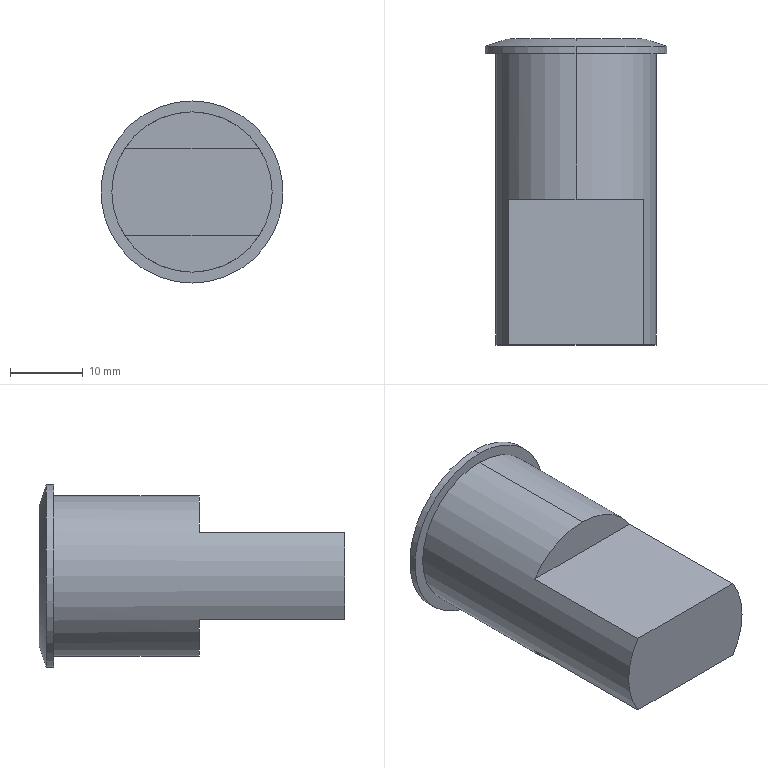Part | SolidWorks | features ICE 2, Chamfer 1, Extrusion 1 | 1 solid | 13 faces | box 25 x 42 x 25 mm | volume 13481 mm3 | plane 7 | cylinder 4 | cone 2 | commonest cylinder face diameters 22 x2 25 x2
STEP:
#1=CARTESIAN_POINT('',(0.,22.,9.5));
#2=VERTEX_POINT('',#1);
#3=CARTESIAN_POINT('',(0.,22.,-9.5));
#4=VERTEX_POINT('',#3);
#5=CARTESIAN_POINT('',(0.,22.,0.));
#6=DIRECTION('',(0.,1.,0.));
#7=DIRECTION('',(0.,0.,1.));
#8=AXIS2_PLACEMENT_3D('',#5,#6,#7);
#9=CIRCLE('',#8,9.5);
#10=EDGE_CURVE('',#2,#4,#9,.T.);
#11=ORIENTED_EDGE('',*,*,#10,.F.);
#12=CARTESIAN_POINT('',(0.,21.,12.5));
#13=VERTEX_POINT('',#12);
#14=CARTESIAN_POINT('',(0.,22.,9.5));
#15=DIRECTION('',(0.,-0.3162,0.9487));
#16=VECTOR('',#15,1000.);
#17=LINE('',#14,#16);
#18=EDGE_CURVE('',#2,#13,#17,.T.);
#19=ORIENTED_EDGE('',*,*,#18,.T.);
#20=CARTESIAN_POINT('',(0.,21.,-12.5));
#21=VERTEX_POINT('',#20);
#22=CARTESIAN_POINT('',(0.,21.,0.));
#23=DIRECTION('',(0.,-1.,0.));
#24=DIRECTION('',(0.,0.,1.));
#25=AXIS2_PLACEMENT_3D('',#22,#23,#24);
#26=CIRCLE('',#25,12.5);
#27=EDGE_CURVE('',#21,#13,#26,.T.);
#28=ORIENTED_EDGE('',*,*,#27,.F.);
#29=CARTESIAN_POINT('',(0.,22.,-9.5));
#30=DIRECTION('',(0.,-0.3162,-0.9487));
#31=VECTOR('',#30,1000.);
#32=LINE('',#29,#31);
#33=EDGE_CURVE('',#4,#21,#32,.T.);
#34=ORIENTED_EDGE('',*,*,#33,.F.);
#35=EDGE_LOOP('',(#11,#19,#28,#34));
#36=FACE_OUTER_BOUND('',#35,.T.);
#37=CARTESIAN_POINT('',(0.,22.,0.));
#38=DIRECTION('',(0.,-1.,0.));
#39=DIRECTION('',(0.,0.,-1.));
#40=AXIS2_PLACEMENT_3D('',#37,#38,#39);
#41=CONICAL_SURFACE('',#40,9.5,1.249);
#42=ADVANCED_FACE('',(#36),#41,.T.);
#43=ORIENTED_EDGE('',*,*,#27,.T.);
#44=CARTESIAN_POINT('',(0.,20.,12.5));
#45=VERTEX_POINT('',#44);
#46=CARTESIAN_POINT('',(0.,22.,12.5));
#47=DIRECTION('',(0.,-1.,0.));
#48=VECTOR('',#47,1000.);
#49=LINE('',#46,#48);
#50=EDGE_CURVE('',#13,#45,#49,.T.);
#51=ORIENTED_EDGE('',*,*,#50,.T.);
#52=CARTESIAN_POINT('',(0.,20.,-12.5));
#53=VERTEX_POINT('',#52);
#54=CARTESIAN_POINT('',(0.,20.,0.));
#55=DIRECTION('',(0.,1.,0.));
#56=DIRECTION('',(0.,0.,1.));
#57=AXIS2_PLACEMENT_3D('',#54,#55,#56);
#58=CIRCLE('',#57,12.5);
#59=EDGE_CURVE('',#45,#53,#58,.T.);
#60=ORIENTED_EDGE('',*,*,#59,.T.);
#61=CARTESIAN_POINT('',(0.,22.,-12.5));
#62=DIRECTION('',(0.,-1.,0.));
#63=VECTOR('',#62,1000.);
#64=LINE('',#61,#63);
#65=EDGE_CURVE('',#21,#53,#64,.T.);
#66=ORIENTED_EDGE('',*,*,#65,.F.);
#67=EDGE_LOOP('',(#43,#51,#60,#66));
#68=FACE_OUTER_BOUND('',#67,.T.);
#69=CARTESIAN_POINT('',(0.,22.,0.));
#70=DIRECTION('',(0.,-1.,0.));
#71=DIRECTION('',(0.,0.,-1.));
#72=AXIS2_PLACEMENT_3D('',#69,#70,#71);
#73=CYLINDRICAL_SURFACE('',#72,12.5);
#74=ADVANCED_FACE('',(#68),#73,.T.);
#75=CARTESIAN_POINT('',(0.,20.,11.));
#76=VERTEX_POINT('',#75);
#77=CARTESIAN_POINT('',(0.,20.,-11.));
#78=VERTEX_POINT('',#77);
#79=CARTESIAN_POINT('',(0.,20.,0.));
#80=DIRECTION('',(0.,1.,0.));
#81=DIRECTION('',(0.,0.,1.));
#82=AXIS2_PLACEMENT_3D('',#79,#80,#81);
#83=CIRCLE('',#82,11.);
#84=EDGE_CURVE('',#76,#78,#83,.T.);
#85=ORIENTED_EDGE('',*,*,#84,.F.);
#86=CARTESIAN_POINT('',(0.,0.,11.));
#87=VERTEX_POINT('',#86);
#88=CARTESIAN_POINT('',(0.,20.,11.));
#89=DIRECTION('',(0.,-1.,0.));
#90=VECTOR('',#89,1000.);
#91=LINE('',#88,#90);
#92=EDGE_CURVE('',#76,#87,#91,.T.);
#93=ORIENTED_EDGE('',*,*,#92,.T.);
#94=CARTESIAN_POINT('',(9.22,0.,6.));
#95=VERTEX_POINT('',#94);
#96=CARTESIAN_POINT('',(0.,0.,0.));
#97=DIRECTION('',(0.,1.,0.));
#98=DIRECTION('',(0.,0.,1.));
#99=AXIS2_PLACEMENT_3D('',#96,#97,#98);
#100=CIRCLE('',#99,11.);
#101=EDGE_CURVE('',#87,#95,#100,.T.);
#102=ORIENTED_EDGE('',*,*,#101,.T.);
#103=CARTESIAN_POINT('',(9.22,-20.,6.));
#104=VERTEX_POINT('',#103);
#105=CARTESIAN_POINT('',(9.22,-20.,6.));
#106=DIRECTION('',(0.,1.,0.));
#107=VECTOR('',#106,1000.);
#108=LINE('',#105,#107);
#109=EDGE_CURVE('',#104,#95,#108,.T.);
#110=ORIENTED_EDGE('',*,*,#109,.F.);
#111=CARTESIAN_POINT('',(9.22,-20.,-6.));
#112=VERTEX_POINT('',#111);
#113=CARTESIAN_POINT('',(0.,-20.,0.));
#114=DIRECTION('',(0.,-1.,0.));
#115=DIRECTION('',(0.,0.,-1.));
#116=AXIS2_PLACEMENT_3D('',#113,#114,#115);
#117=CIRCLE('',#116,11.);
#118=EDGE_CURVE('',#112,#104,#117,.T.);
#119=ORIENTED_EDGE('',*,*,#118,.F.);
#120=CARTESIAN_POINT('',(9.22,0.,-6.));
#121=VERTEX_POINT('',#120);
#122=CARTESIAN_POINT('',(9.22,-20.,-6.));
#123=DIRECTION('',(0.,1.,0.));
#124=VECTOR('',#123,1000.);
#125=LINE('',#122,#124);
#126=EDGE_CURVE('',#112,#121,#125,.T.);
#127=ORIENTED_EDGE('',*,*,#126,.T.);
#128=CARTESIAN_POINT('',(0.,0.,-11.));
#129=VERTEX_POINT('',#128);
#130=CARTESIAN_POINT('',(0.,0.,0.));
#131=DIRECTION('',(0.,1.,0.));
#132=DIRECTION('',(0.,0.,1.));
#133=AXIS2_PLACEMENT_3D('',#130,#131,#132);
#134=CIRCLE('',#133,11.);
#135=EDGE_CURVE('',#121,#129,#134,.T.);
#136=ORIENTED_EDGE('',*,*,#135,.T.);
#137=CARTESIAN_POINT('',(0.,20.,-11.));
#138=DIRECTION('',(0.,-1.,0.));
#139=VECTOR('',#138,1000.);
#140=LINE('',#137,#139);
#141=EDGE_CURVE('',#78,#129,#140,.T.);
#142=ORIENTED_EDGE('',*,*,#141,.F.);
#143=EDGE_LOOP('',(#85,#93,#102,#110,#119,#127,#136,#142));
#144=FACE_OUTER_BOUND('',#143,.T.);
#145=CARTESIAN_POINT('',(0.,20.,0.));
#146=DIRECTION('',(0.,-1.,0.));
#147=DIRECTION('',(0.,0.,-1.));
#148=AXIS2_PLACEMENT_3D('',#145,#146,#147);
#149=CYLINDRICAL_SURFACE('',#148,11.);
#150=ADVANCED_FACE('',(#144),#149,.T.);
#151=CARTESIAN_POINT('',(-9.22,0.,-6.));
#152=VERTEX_POINT('',#151);
#153=CARTESIAN_POINT('',(0.,0.,-6.));
#154=DIRECTION('',(1.,0.,0.));
#155=VECTOR('',#154,1000.);
#156=LINE('',#153,#155);
#157=EDGE_CURVE('',#152,#121,#156,.T.);
#158=ORIENTED_EDGE('',*,*,#157,.F.);
#159=CARTESIAN_POINT('',(0.,0.,0.));
#160=DIRECTION('',(0.,1.,0.));
#161=DIRECTION('',(0.,0.,1.));
#162=AXIS2_PLACEMENT_3D('',#159,#160,#161);
#163=CIRCLE('',#162,11.);
#164=EDGE_CURVE('',#129,#152,#163,.T.);
#165=ORIENTED_EDGE('',*,*,#164,.F.);
#166=ORIENTED_EDGE('',*,*,#135,.F.);
#167=EDGE_LOOP('',(#158,#165,#166));
#168=FACE_OUTER_BOUND('',#167,.T.);
#169=CARTESIAN_POINT('',(0.,0.,0.));
#170=DIRECTION('',(0.,1.,0.));
#171=DIRECTION('',(0.,0.,1.));
#172=AXIS2_PLACEMENT_3D('',#169,#170,#171);
#173=PLANE('',#172);
#174=ADVANCED_FACE('',(#168),#173,.F.);
#175=ORIENTED_EDGE('',*,*,#92,.F.);
#176=CARTESIAN_POINT('',(0.,20.,0.));
#177=DIRECTION('',(0.,1.,0.));
#178=DIRECTION('',(0.,0.,1.));
#179=AXIS2_PLACEMENT_3D('',#176,#177,#178);
#180=CIRCLE('',#179,11.);
#181=EDGE_CURVE('',#78,#76,#180,.T.);
#182=ORIENTED_EDGE('',*,*,#181,.F.);
#183=ORIENTED_EDGE('',*,*,#141,.T.);
#184=ORIENTED_EDGE('',*,*,#164,.T.);
#185=CARTESIAN_POINT('',(-9.22,-20.,-6.));
#186=VERTEX_POINT('',#185);
#187=CARTESIAN_POINT('',(-9.22,-20.,-6.));
#188=DIRECTION('',(0.,1.,0.));
#189=VECTOR('',#188,1000.);
#190=LINE('',#187,#189);
#191=EDGE_CURVE('',#186,#152,#190,.T.);
#192=ORIENTED_EDGE('',*,*,#191,.F.);
#193=CARTESIAN_POINT('',(-9.22,-20.,6.));
#194=VERTEX_POINT('',#193);
#195=CARTESIAN_POINT('',(0.,-20.,0.));
#196=DIRECTION('',(0.,-1.,0.));
#197=DIRECTION('',(0.,0.,-1.));
#198=AXIS2_PLACEMENT_3D('',#195,#196,#197);
#199=CIRCLE('',#198,11.);
#200=EDGE_CURVE('',#194,#186,#199,.T.);
#201=ORIENTED_EDGE('',*,*,#200,.F.);
#202=CARTESIAN_POINT('',(-9.22,0.,6.));
#203=VERTEX_POINT('',#202);
#204=CARTESIAN_POINT('',(-9.22,-20.,6.));
#205=DIRECTION('',(0.,1.,0.));
#206=VECTOR('',#205,1000.);
#207=LINE('',#204,#206);
#208=EDGE_CURVE('',#194,#203,#207,.T.);
#209=ORIENTED_EDGE('',*,*,#208,.T.);
#210=CARTESIAN_POINT('',(0.,0.,0.));
#211=DIRECTION('',(0.,1.,0.));
#212=DIRECTION('',(0.,0.,1.));
#213=AXIS2_PLACEMENT_3D('',#210,#211,#212);
#214=CIRCLE('',#213,11.);
#215=EDGE_CURVE('',#203,#87,#214,.T.);
#216=ORIENTED_EDGE('',*,*,#215,.T.);
#217=EDGE_LOOP('',(#175,#182,#183,#184,#192,#201,#209,#216));
#218=FACE_OUTER_BOUND('',#217,.T.);
#219=CARTESIAN_POINT('',(0.,20.,0.));
#220=DIRECTION('',(0.,-1.,0.));
#221=DIRECTION('',(0.,0.,-1.));
#222=AXIS2_PLACEMENT_3D('',#219,#220,#221);
#223=CYLINDRICAL_SURFACE('',#222,11.);
#224=ADVANCED_FACE('',(#218),#223,.T.);
#225=ORIENTED_EDGE('',*,*,#215,.F.);
#226=CARTESIAN_POINT('',(0.,0.,6.));
#227=DIRECTION('',(1.,0.,0.));
#228=VECTOR('',#227,1000.);
#229=LINE('',#226,#228);
#230=EDGE_CURVE('',#203,#95,#229,.T.);
#231=ORIENTED_EDGE('',*,*,#230,.T.);
#232=ORIENTED_EDGE('',*,*,#101,.F.);
#233=EDGE_LOOP('',(#225,#231,#232));
#234=FACE_OUTER_BOUND('',#233,.T.);
#235=CARTESIAN_POINT('',(0.,0.,0.));
#236=DIRECTION('',(0.,1.,0.));
#237=DIRECTION('',(0.,0.,1.));
#238=AXIS2_PLACEMENT_3D('',#235,#236,#237);
#239=PLANE('',#238);
#240=ADVANCED_FACE('',(#234),#239,.F.);
#241=ORIENTED_EDGE('',*,*,#157,.T.);
#242=ORIENTED_EDGE('',*,*,#126,.F.);
#243=CARTESIAN_POINT('',(0.,-20.,-6.));
#244=DIRECTION('',(1.,0.,0.));
#245=VECTOR('',#244,1000.);
#246=LINE('',#243,#245);
#247=EDGE_CURVE('',#186,#112,#246,.T.);
#248=ORIENTED_EDGE('',*,*,#247,.F.);
#249=ORIENTED_EDGE('',*,*,#191,.T.);
#250=EDGE_LOOP('',(#241,#242,#248,#249));
#251=FACE_OUTER_BOUND('',#250,.T.);
#252=CARTESIAN_POINT('',(0.,-20.,-6.));
#253=DIRECTION('',(0.,0.,1.));
#254=DIRECTION('',(1.,0.,0.));
#255=AXIS2_PLACEMENT_3D('',#252,#253,#254);
#256=PLANE('',#255);
#257=ADVANCED_FACE('',(#251),#256,.F.);
#258=ORIENTED_EDGE('',*,*,#230,.F.);
#259=ORIENTED_EDGE('',*,*,#208,.F.);
#260=CARTESIAN_POINT('',(0.,-20.,6.));
#261=DIRECTION('',(1.,0.,0.));
#262=VECTOR('',#261,1000.);
#263=LINE('',#260,#262);
#264=EDGE_CURVE('',#194,#104,#263,.T.);
#265=ORIENTED_EDGE('',*,*,#264,.T.);
#266=ORIENTED_EDGE('',*,*,#109,.T.);
#267=EDGE_LOOP('',(#258,#259,#265,#266));
#268=FACE_OUTER_BOUND('',#267,.T.);
#269=CARTESIAN_POINT('',(0.,-20.,6.));
#270=DIRECTION('',(0.,0.,1.));
#271=DIRECTION('',(1.,0.,0.));
#272=AXIS2_PLACEMENT_3D('',#269,#270,#271);
#273=PLANE('',#272);
#274=ADVANCED_FACE('',(#268),#273,.T.);
#275=ORIENTED_EDGE('',*,*,#200,.T.);
#276=ORIENTED_EDGE('',*,*,#247,.T.);
#277=ORIENTED_EDGE('',*,*,#118,.T.);
#278=ORIENTED_EDGE('',*,*,#264,.F.);
#279=EDGE_LOOP('',(#275,#276,#277,#278));
#280=FACE_OUTER_BOUND('',#279,.T.);
#281=CARTESIAN_POINT('',(0.,-20.,0.));
#282=DIRECTION('',(0.,-1.,0.));
#283=DIRECTION('',(0.,0.,-1.));
#284=AXIS2_PLACEMENT_3D('',#281,#282,#283);
#285=PLANE('',#284);
#286=ADVANCED_FACE('',(#280),#285,.T.);
#287=ORIENTED_EDGE('',*,*,#50,.F.);
#288=CARTESIAN_POINT('',(0.,21.,0.));
#289=DIRECTION('',(0.,-1.,0.));
#290=DIRECTION('',(0.,0.,1.));
#291=AXIS2_PLACEMENT_3D('',#288,#289,#290);
#292=CIRCLE('',#291,12.5);
#293=EDGE_CURVE('',#13,#21,#292,.T.);
#294=ORIENTED_EDGE('',*,*,#293,.T.);
#295=ORIENTED_EDGE('',*,*,#65,.T.);
#296=CARTESIAN_POINT('',(0.,20.,0.));
#297=DIRECTION('',(0.,1.,0.));
#298=DIRECTION('',(0.,0.,1.));
#299=AXIS2_PLACEMENT_3D('',#296,#297,#298);
#300=CIRCLE('',#299,12.5);
#301=EDGE_CURVE('',#53,#45,#300,.T.);
#302=ORIENTED_EDGE('',*,*,#301,.T.);
#303=EDGE_LOOP('',(#287,#294,#295,#302));
#304=FACE_OUTER_BOUND('',#303,.T.);
#305=CARTESIAN_POINT('',(0.,22.,0.));
#306=DIRECTION('',(0.,-1.,0.));
#307=DIRECTION('',(0.,0.,-1.));
#308=AXIS2_PLACEMENT_3D('',#305,#306,#307);
#309=CYLINDRICAL_SURFACE('',#308,12.5);
#310=ADVANCED_FACE('',(#304),#309,.T.);
#311=CARTESIAN_POINT('',(0.,22.,0.));
#312=DIRECTION('',(0.,1.,0.));
#313=DIRECTION('',(0.,0.,1.));
#314=AXIS2_PLACEMENT_3D('',#311,#312,#313);
#315=CIRCLE('',#314,9.5);
#316=EDGE_CURVE('',#4,#2,#315,.T.);
#317=ORIENTED_EDGE('',*,*,#316,.T.);
#318=ORIENTED_EDGE('',*,*,#10,.T.);
#319=EDGE_LOOP('',(#317,#318));
#320=FACE_OUTER_BOUND('',#319,.T.);
#321=CARTESIAN_POINT('',(0.,22.,0.));
#322=DIRECTION('',(0.,1.,0.));
#323=DIRECTION('',(0.,0.,1.));
#324=AXIS2_PLACEMENT_3D('',#321,#322,#323);
#325=PLANE('',#324);
#326=ADVANCED_FACE('',(#320),#325,.T.);
#327=ORIENTED_EDGE('',*,*,#181,.T.);
#328=ORIENTED_EDGE('',*,*,#84,.T.);
#329=EDGE_LOOP('',(#327,#328));
#330=FACE_BOUND('',#329,.T.);
#331=ORIENTED_EDGE('',*,*,#301,.F.);
#332=ORIENTED_EDGE('',*,*,#59,.F.);
#333=EDGE_LOOP('',(#331,#332));
#334=FACE_OUTER_BOUND('',#333,.T.);
#335=CARTESIAN_POINT('',(0.,20.,0.));
#336=DIRECTION('',(0.,1.,0.));
#337=DIRECTION('',(0.,0.,1.));
#338=AXIS2_PLACEMENT_3D('',#335,#336,#337);
#339=PLANE('',#338);
#340=ADVANCED_FACE('',(#330,#334),#339,.F.);
#341=ORIENTED_EDGE('',*,*,#18,.F.);
#342=ORIENTED_EDGE('',*,*,#316,.F.);
#343=ORIENTED_EDGE('',*,*,#33,.T.);
#344=ORIENTED_EDGE('',*,*,#293,.F.);
#345=EDGE_LOOP('',(#341,#342,#343,#344));
#346=FACE_OUTER_BOUND('',#345,.T.);
#347=CARTESIAN_POINT('',(0.,22.,0.));
#348=DIRECTION('',(0.,-1.,0.));
#349=DIRECTION('',(0.,0.,-1.));
#350=AXIS2_PLACEMENT_3D('',#347,#348,#349);
#351=CONICAL_SURFACE('',#350,9.5,1.249);
#352=ADVANCED_FACE('',(#346),#351,.T.);
#353=CLOSED_SHELL('',(#42,#74,#150,#174,#224,#240,#257,#274,#286,#310,#326,#340,#352));
#354=MANIFOLD_SOLID_BREP('',#353);
#355=CARTESIAN_POINT('',(0.,0.,0.));
#356=DIRECTION('',(0.,0.,1.));
#357=DIRECTION('',(1.,0.,0.));
#358=AXIS2_PLACEMENT_3D('',#355,#356,#357);
#359=(LENGTH_UNIT()NAMED_UNIT(*)SI_UNIT(.MILLI.,.METRE.));
#360=UNCERTAINTY_MEASURE_WITH_UNIT(LENGTH_MEASURE(0.00001),#359,'','');
#361=(NAMED_UNIT(*)PLANE_ANGLE_UNIT()SI_UNIT($,.RADIAN.));
#362=(NAMED_UNIT(*)SI_UNIT($,.STERADIAN.)SOLID_ANGLE_UNIT());
#363=(GEOMETRIC_REPRESENTATION_CONTEXT(3)GLOBAL_UNCERTAINTY_ASSIGNED_CONTEXT((#360))GLOBAL_UNIT_ASSIGNED_CONTEXT((#359,#361,#362))REPRESENTATION_CONTEXT('',''));
#364=ADVANCED_BREP_SHAPE_REPRESENTATION('',(#354,#358),#363);